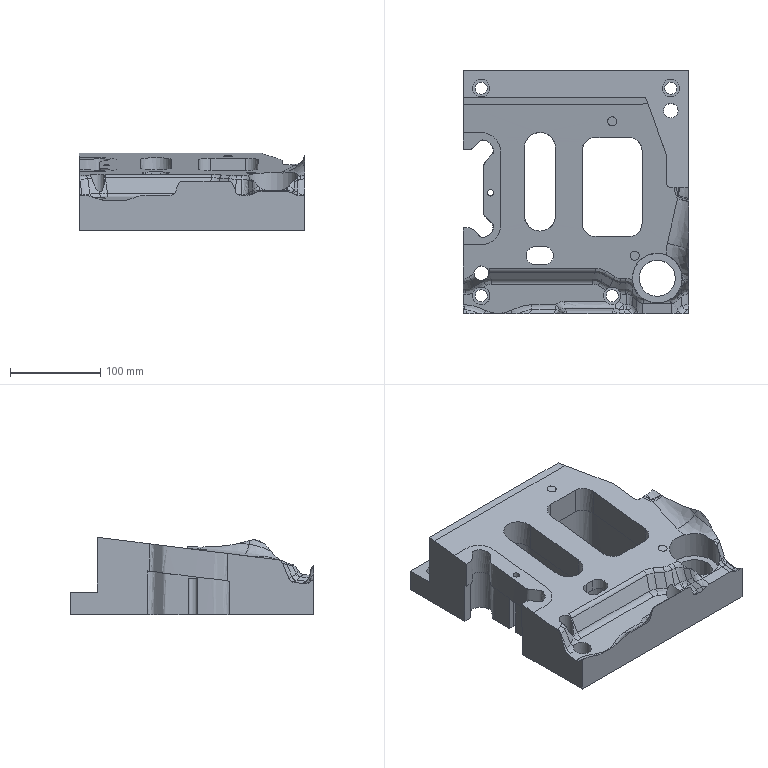Part | NX | features solid 2 | 1 solid | 185 faces | box 250.006 x 270.004 x 85.748 mm | volume 2833061 mm3 | spline 139 | plane 28 | cylinder 18 | commonest cylinder face diameters 13.5 x4 19.5 x4 10 x2 16 x2 20 x2 7 x1